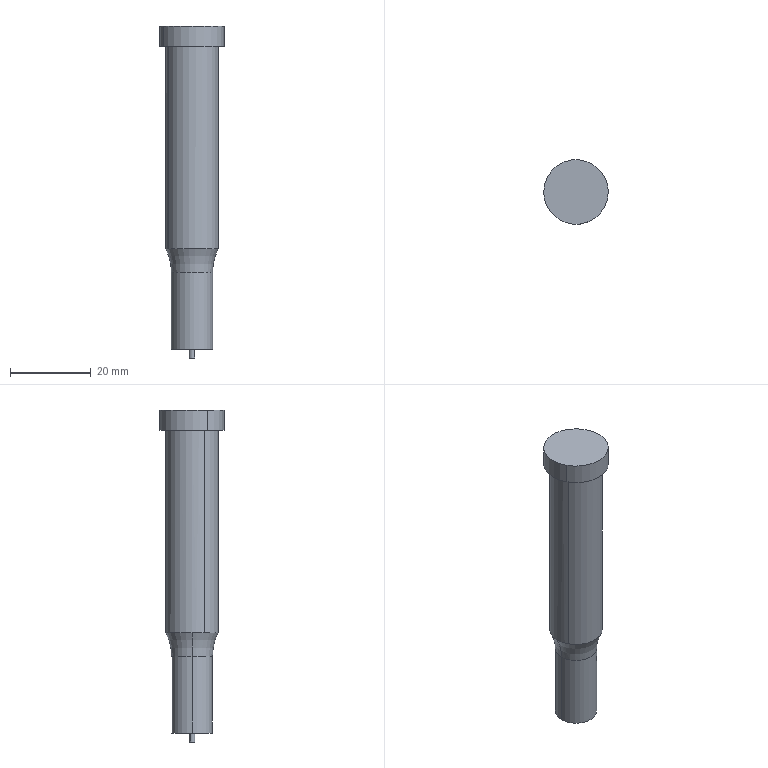Part | CATIA | 1 solid | 14 faces | box 16 x 16 x 82.2 mm | volume 9788 mm3 | cylinder 8 | plane 4 | torus 2 | commonest cylinder face diameters 1.47 x2 10.2 x2 13 x2 16 x2
STEP:
#1=CARTESIAN_POINT('',(5.1,0.,0.));
#2=VERTEX_POINT('',#1);
#3=CARTESIAN_POINT('',(-5.1,0.,0.));
#4=VERTEX_POINT('',#3);
#5=CARTESIAN_POINT('',(0.,0.,0.));
#6=DIRECTION('',(0.,0.,1.));
#7=AXIS2_PLACEMENT_3D('',#5,#6,$);
#8=CIRCLE('',#7,5.1);
#9=EDGE_CURVE('',#2,#4,#8,.T.);
#10=ORIENTED_EDGE('',*,*,#9,.F.);
#11=CARTESIAN_POINT('',(0.,0.,0.));
#12=DIRECTION('',(0.,0.,1.));
#13=AXIS2_PLACEMENT_3D('',#11,#12,$);
#14=CIRCLE('',#13,5.1);
#15=EDGE_CURVE('',#4,#2,#14,.T.);
#16=ORIENTED_EDGE('',*,*,#15,.F.);
#17=EDGE_LOOP('',(#10,#16));
#18=FACE_OUTER_BOUND('',#17,.T.);
#19=CARTESIAN_POINT('',(0.645,-0.3524,0.));
#20=VERTEX_POINT('',#19);
#21=CARTESIAN_POINT('',(-0.645,0.3524,0.));
#22=VERTEX_POINT('',#21);
#23=CARTESIAN_POINT('',(0.,0.,0.));
#24=DIRECTION('',(0.,0.,1.));
#25=AXIS2_PLACEMENT_3D('',#23,#24,$);
#26=CIRCLE('',#25,0.735);
#27=EDGE_CURVE('',#20,#22,#26,.F.);
#28=ORIENTED_EDGE('',*,*,#27,.F.);
#29=CARTESIAN_POINT('',(0.,0.,0.));
#30=DIRECTION('',(0.,0.,1.));
#31=AXIS2_PLACEMENT_3D('',#29,#30,$);
#32=CIRCLE('',#31,0.735);
#33=EDGE_CURVE('',#22,#20,#32,.F.);
#34=ORIENTED_EDGE('',*,*,#33,.F.);
#35=EDGE_LOOP('',(#28,#34));
#36=FACE_BOUND('',#35,.T.);
#37=CARTESIAN_POINT('',(6.5,0.,0.));
#38=DIRECTION('',(0.,0.,1.));
#39=DIRECTION('',(1.,0.,0.));
#40=AXIS2_PLACEMENT_3D('',#37,#38,#39);
#41=PLANE('',#40);
#42=ADVANCED_FACE('',(#18,#36),#41,.F.);
#43=CARTESIAN_POINT('',(-6.5,0.,24.869));
#44=VERTEX_POINT('',#43);
#45=CARTESIAN_POINT('',(5.704,3.116,24.869));
#46=VERTEX_POINT('',#45);
#47=CARTESIAN_POINT('',(0.,0.,24.869));
#48=DIRECTION('',(0.,0.,-1.));
#49=AXIS2_PLACEMENT_3D('',#47,#48,$);
#50=CIRCLE('',#49,6.5);
#51=EDGE_CURVE('',#44,#46,#50,.T.);
#52=ORIENTED_EDGE('',*,*,#51,.T.);
#53=CARTESIAN_POINT('',(6.5,0.,24.869));
#54=VERTEX_POINT('',#53);
#55=CARTESIAN_POINT('',(0.,0.,24.869));
#56=DIRECTION('',(0.,0.,-1.));
#57=AXIS2_PLACEMENT_3D('',#55,#56,$);
#58=CIRCLE('',#57,6.5);
#59=EDGE_CURVE('',#46,#54,#58,.T.);
#60=ORIENTED_EDGE('',*,*,#59,.T.);
#61=CARTESIAN_POINT('',(5.1,0.,19.));
#62=VERTEX_POINT('',#61);
#63=CARTESIAN_POINT('',(18.1,0.,19.));
#64=DIRECTION('',(0.,1.,0.));
#65=AXIS2_PLACEMENT_3D('',#63,#64,$);
#66=CIRCLE('',#65,13.);
#67=EDGE_CURVE('',#54,#62,#66,.F.);
#68=ORIENTED_EDGE('',*,*,#67,.T.);
#69=CARTESIAN_POINT('',(-5.1,0.,19.));
#70=VERTEX_POINT('',#69);
#71=CARTESIAN_POINT('',(0.,0.,19.));
#72=DIRECTION('',(0.,0.,-1.));
#73=AXIS2_PLACEMENT_3D('',#71,#72,$);
#74=CIRCLE('',#73,5.1);
#75=EDGE_CURVE('',#70,#62,#74,.T.);
#76=ORIENTED_EDGE('',*,*,#75,.F.);
#77=CARTESIAN_POINT('',(-18.1,0.,19.));
#78=DIRECTION('',(0.,-1.,0.));
#79=AXIS2_PLACEMENT_3D('',#77,#78,$);
#80=CIRCLE('',#79,13.);
#81=EDGE_CURVE('',#44,#70,#80,.F.);
#82=ORIENTED_EDGE('',*,*,#81,.F.);
#83=EDGE_LOOP('',(#52,#60,#68,#76,#82));
#84=FACE_OUTER_BOUND('',#83,.T.);
#85=CARTESIAN_POINT('',(0.,0.,19.));
#86=DIRECTION('',(0.,0.,-1.));
#87=DIRECTION('',(-0.9236,-0.3833,0.));
#88=AXIS2_PLACEMENT_3D('',#85,#86,#87);
#89=TOROIDAL_SURFACE('',#88,18.1,13.);
#90=ADVANCED_FACE('',(#84),#89,.F.);
#91=CARTESIAN_POINT('',(-5.704,-3.116,24.869));
#92=VERTEX_POINT('',#91);
#93=CARTESIAN_POINT('',(0.,0.,24.869));
#94=DIRECTION('',(0.,0.,-1.));
#95=AXIS2_PLACEMENT_3D('',#93,#94,$);
#96=CIRCLE('',#95,6.5);
#97=EDGE_CURVE('',#92,#54,#96,.F.);
#98=ORIENTED_EDGE('',*,*,#97,.F.);
#99=CARTESIAN_POINT('',(0.,0.,24.869));
#100=DIRECTION('',(0.,0.,-1.));
#101=AXIS2_PLACEMENT_3D('',#99,#100,$);
#102=CIRCLE('',#101,6.5);
#103=EDGE_CURVE('',#92,#44,#102,.T.);
#104=ORIENTED_EDGE('',*,*,#103,.T.);
#105=ORIENTED_EDGE('',*,*,#81,.T.);
#106=CARTESIAN_POINT('',(0.,0.,19.));
#107=DIRECTION('',(0.,0.,-1.));
#108=AXIS2_PLACEMENT_3D('',#106,#107,$);
#109=CIRCLE('',#108,5.1);
#110=EDGE_CURVE('',#62,#70,#109,.T.);
#111=ORIENTED_EDGE('',*,*,#110,.F.);
#112=ORIENTED_EDGE('',*,*,#67,.F.);
#113=EDGE_LOOP('',(#98,#104,#105,#111,#112));
#114=FACE_OUTER_BOUND('',#113,.T.);
#115=CARTESIAN_POINT('',(0.,0.,19.));
#116=DIRECTION('',(0.,0.,-1.));
#117=DIRECTION('',(0.9063,0.4226,0.));
#118=AXIS2_PLACEMENT_3D('',#115,#116,#117);
#119=TOROIDAL_SURFACE('',#118,18.1,13.);
#120=ADVANCED_FACE('',(#114),#119,.F.);
#121=CARTESIAN_POINT('',(5.1,0.,16.61));
#122=DIRECTION('',(0.,0.,1.));
#123=VECTOR('',#122,1.);
#124=LINE('',#121,#123);
#125=EDGE_CURVE('',#2,#62,#124,.T.);
#126=ORIENTED_EDGE('',*,*,#125,.F.);
#127=ORIENTED_EDGE('',*,*,#9,.T.);
#128=CARTESIAN_POINT('',(-5.1,0.,16.61));
#129=DIRECTION('',(0.,0.,1.));
#130=VECTOR('',#129,1.);
#131=LINE('',#128,#130);
#132=EDGE_CURVE('',#4,#70,#131,.T.);
#133=ORIENTED_EDGE('',*,*,#132,.T.);
#134=ORIENTED_EDGE('',*,*,#75,.T.);
#135=EDGE_LOOP('',(#126,#127,#133,#134));
#136=FACE_OUTER_BOUND('',#135,.T.);
#137=CARTESIAN_POINT('',(0.,0.,16.61));
#138=DIRECTION('',(0.,0.,1.));
#139=DIRECTION('',(1.,0.,0.));
#140=AXIS2_PLACEMENT_3D('',#137,#138,#139);
#141=CYLINDRICAL_SURFACE('',#140,5.1);
#142=ADVANCED_FACE('',(#136),#141,.T.);
#143=ORIENTED_EDGE('',*,*,#132,.F.);
#144=ORIENTED_EDGE('',*,*,#15,.T.);
#145=ORIENTED_EDGE('',*,*,#125,.T.);
#146=ORIENTED_EDGE('',*,*,#110,.T.);
#147=EDGE_LOOP('',(#143,#144,#145,#146));
#148=FACE_OUTER_BOUND('',#147,.T.);
#149=CARTESIAN_POINT('',(0.,0.,16.61));
#150=DIRECTION('',(0.,0.,1.));
#151=DIRECTION('',(-1.,0.,0.));
#152=AXIS2_PLACEMENT_3D('',#149,#150,#151);
#153=CYLINDRICAL_SURFACE('',#152,5.1);
#154=ADVANCED_FACE('',(#148),#153,.T.);
#155=CARTESIAN_POINT('',(-5.704,-3.116,75.));
#156=VERTEX_POINT('',#155);
#157=CARTESIAN_POINT('',(-5.704,-3.116,37.5));
#158=DIRECTION('',(0.,0.,1.));
#159=VECTOR('',#158,1.);
#160=LINE('',#157,#159);
#161=EDGE_CURVE('',#92,#156,#160,.T.);
#162=ORIENTED_EDGE('',*,*,#161,.T.);
#163=CARTESIAN_POINT('',(5.704,3.116,75.));
#164=VERTEX_POINT('',#163);
#165=CARTESIAN_POINT('',(0.,0.,75.));
#166=DIRECTION('',(0.,0.,1.));
#167=AXIS2_PLACEMENT_3D('',#165,#166,$);
#168=CIRCLE('',#167,6.5);
#169=EDGE_CURVE('',#164,#156,#168,.T.);
#170=ORIENTED_EDGE('',*,*,#169,.F.);
#171=CARTESIAN_POINT('',(5.704,3.116,37.5));
#172=DIRECTION('',(0.,0.,1.));
#173=VECTOR('',#172,1.);
#174=LINE('',#171,#173);
#175=EDGE_CURVE('',#46,#164,#174,.T.);
#176=ORIENTED_EDGE('',*,*,#175,.F.);
#177=ORIENTED_EDGE('',*,*,#51,.F.);
#178=ORIENTED_EDGE('',*,*,#103,.F.);
#179=EDGE_LOOP('',(#162,#170,#176,#177,#178));
#180=FACE_OUTER_BOUND('',#179,.T.);
#181=CARTESIAN_POINT('',(0.,0.,40.));
#182=DIRECTION('',(0.,0.,1.));
#183=DIRECTION('',(0.8776,0.4794,0.));
#184=AXIS2_PLACEMENT_3D('',#181,#182,#183);
#185=CYLINDRICAL_SURFACE('',#184,6.5);
#186=ADVANCED_FACE('',(#180),#185,.T.);
#187=ORIENTED_EDGE('',*,*,#175,.T.);
#188=CARTESIAN_POINT('',(0.,0.,75.));
#189=DIRECTION('',(0.,0.,1.));
#190=AXIS2_PLACEMENT_3D('',#188,#189,$);
#191=CIRCLE('',#190,6.5);
#192=EDGE_CURVE('',#156,#164,#191,.T.);
#193=ORIENTED_EDGE('',*,*,#192,.F.);
#194=ORIENTED_EDGE('',*,*,#161,.F.);
#195=ORIENTED_EDGE('',*,*,#97,.T.);
#196=ORIENTED_EDGE('',*,*,#59,.F.);
#197=EDGE_LOOP('',(#187,#193,#194,#195,#196));
#198=FACE_OUTER_BOUND('',#197,.T.);
#199=ADVANCED_FACE('',(#198),#185,.T.);
#200=CARTESIAN_POINT('',(-7.021,-3.835,80.));
#201=VERTEX_POINT('',#200);
#202=CARTESIAN_POINT('',(7.021,3.835,80.));
#203=VERTEX_POINT('',#202);
#204=CARTESIAN_POINT('',(0.,0.,80.));
#205=DIRECTION('',(0.,0.,1.));
#206=AXIS2_PLACEMENT_3D('',#204,#205,$);
#207=CIRCLE('',#206,8.);
#208=EDGE_CURVE('',#201,#203,#207,.T.);
#209=ORIENTED_EDGE('',*,*,#208,.T.);
#210=CARTESIAN_POINT('',(0.,0.,80.));
#211=DIRECTION('',(0.,0.,1.));
#212=AXIS2_PLACEMENT_3D('',#210,#211,$);
#213=CIRCLE('',#212,8.);
#214=EDGE_CURVE('',#203,#201,#213,.T.);
#215=ORIENTED_EDGE('',*,*,#214,.T.);
#216=EDGE_LOOP('',(#209,#215));
#217=FACE_OUTER_BOUND('',#216,.T.);
#218=CARTESIAN_POINT('',(0.,0.,80.));
#219=DIRECTION('',(0.,0.,1.));
#220=DIRECTION('',(1.,0.,0.));
#221=AXIS2_PLACEMENT_3D('',#218,#219,#220);
#222=PLANE('',#221);
#223=ADVANCED_FACE('',(#217),#222,.T.);
#224=CARTESIAN_POINT('',(7.021,3.835,75.));
#225=VERTEX_POINT('',#224);
#226=CARTESIAN_POINT('',(-7.021,-3.835,75.));
#227=VERTEX_POINT('',#226);
#228=CARTESIAN_POINT('',(0.,0.,75.));
#229=DIRECTION('',(0.,0.,1.));
#230=AXIS2_PLACEMENT_3D('',#228,#229,$);
#231=CIRCLE('',#230,8.);
#232=EDGE_CURVE('',#225,#227,#231,.T.);
#233=ORIENTED_EDGE('',*,*,#232,.F.);
#234=CARTESIAN_POINT('',(0.,0.,75.));
#235=DIRECTION('',(0.,0.,1.));
#236=AXIS2_PLACEMENT_3D('',#234,#235,$);
#237=CIRCLE('',#236,8.);
#238=EDGE_CURVE('',#227,#225,#237,.T.);
#239=ORIENTED_EDGE('',*,*,#238,.F.);
#240=EDGE_LOOP('',(#233,#239));
#241=FACE_OUTER_BOUND('',#240,.T.);
#242=ORIENTED_EDGE('',*,*,#192,.T.);
#243=ORIENTED_EDGE('',*,*,#169,.T.);
#244=EDGE_LOOP('',(#242,#243));
#245=FACE_BOUND('',#244,.T.);
#246=CARTESIAN_POINT('',(8.,0.,75.));
#247=DIRECTION('',(0.,0.,1.));
#248=DIRECTION('',(1.,0.,0.));
#249=AXIS2_PLACEMENT_3D('',#246,#247,#248);
#250=PLANE('',#249);
#251=ADVANCED_FACE('',(#241,#245),#250,.F.);
#252=CARTESIAN_POINT('',(7.021,3.835,77.5));
#253=DIRECTION('',(0.,0.,1.));
#254=VECTOR('',#253,1.);
#255=LINE('',#252,#254);
#256=EDGE_CURVE('',#225,#203,#255,.T.);
#257=ORIENTED_EDGE('',*,*,#256,.T.);
#258=ORIENTED_EDGE('',*,*,#208,.F.);
#259=CARTESIAN_POINT('',(-7.021,-3.835,77.5));
#260=DIRECTION('',(0.,0.,1.));
#261=VECTOR('',#260,1.);
#262=LINE('',#259,#261);
#263=EDGE_CURVE('',#227,#201,#262,.T.);
#264=ORIENTED_EDGE('',*,*,#263,.F.);
#265=ORIENTED_EDGE('',*,*,#238,.T.);
#266=EDGE_LOOP('',(#257,#258,#264,#265));
#267=FACE_OUTER_BOUND('',#266,.T.);
#268=CARTESIAN_POINT('',(0.,0.,40.));
#269=DIRECTION('',(0.,0.,1.));
#270=DIRECTION('',(0.8776,0.4794,0.));
#271=AXIS2_PLACEMENT_3D('',#268,#269,#270);
#272=CYLINDRICAL_SURFACE('',#271,8.);
#273=ADVANCED_FACE('',(#267),#272,.T.);
#274=ORIENTED_EDGE('',*,*,#263,.T.);
#275=ORIENTED_EDGE('',*,*,#214,.F.);
#276=ORIENTED_EDGE('',*,*,#256,.F.);
#277=ORIENTED_EDGE('',*,*,#232,.T.);
#278=EDGE_LOOP('',(#274,#275,#276,#277));
#279=FACE_OUTER_BOUND('',#278,.T.);
#280=ADVANCED_FACE('',(#279),#272,.T.);
#281=CARTESIAN_POINT('',(0.645,-0.3524,-2.2));
#282=VERTEX_POINT('',#281);
#283=CARTESIAN_POINT('',(-0.645,0.3524,-2.2));
#284=VERTEX_POINT('',#283);
#285=CARTESIAN_POINT('',(0.,0.,-2.2));
#286=DIRECTION('',(0.,0.,-1.));
#287=AXIS2_PLACEMENT_3D('',#285,#286,$);
#288=CIRCLE('',#287,0.735);
#289=EDGE_CURVE('',#282,#284,#288,.T.);
#290=ORIENTED_EDGE('',*,*,#289,.F.);
#291=CARTESIAN_POINT('',(0.645,-0.3524,-1.1));
#292=DIRECTION('',(0.,0.,-1.));
#293=VECTOR('',#292,1.);
#294=LINE('',#291,#293);
#295=EDGE_CURVE('',#282,#20,#294,.F.);
#296=ORIENTED_EDGE('',*,*,#295,.T.);
#297=ORIENTED_EDGE('',*,*,#27,.T.);
#298=CARTESIAN_POINT('',(-0.645,0.3524,-1.1));
#299=DIRECTION('',(0.,0.,-1.));
#300=VECTOR('',#299,1.);
#301=LINE('',#298,#300);
#302=EDGE_CURVE('',#284,#22,#301,.F.);
#303=ORIENTED_EDGE('',*,*,#302,.F.);
#304=EDGE_LOOP('',(#290,#296,#297,#303));
#305=FACE_OUTER_BOUND('',#304,.T.);
#306=CARTESIAN_POINT('',(0.,0.,-1.1));
#307=DIRECTION('',(0.,0.,-1.));
#308=DIRECTION('',(0.8776,-0.4794,0.));
#309=AXIS2_PLACEMENT_3D('',#306,#307,#308);
#310=CYLINDRICAL_SURFACE('',#309,0.735);
#311=ADVANCED_FACE('',(#305),#310,.T.);
#312=CARTESIAN_POINT('',(0.,0.,-2.2));
#313=DIRECTION('',(0.,0.,-1.));
#314=AXIS2_PLACEMENT_3D('',#312,#313,$);
#315=CIRCLE('',#314,0.735);
#316=EDGE_CURVE('',#284,#282,#315,.T.);
#317=ORIENTED_EDGE('',*,*,#316,.F.);
#318=ORIENTED_EDGE('',*,*,#302,.T.);
#319=ORIENTED_EDGE('',*,*,#33,.T.);
#320=ORIENTED_EDGE('',*,*,#295,.F.);
#321=EDGE_LOOP('',(#317,#318,#319,#320));
#322=FACE_OUTER_BOUND('',#321,.T.);
#323=ADVANCED_FACE('',(#322),#310,.T.);
#324=ORIENTED_EDGE('',*,*,#289,.T.);
#325=ORIENTED_EDGE('',*,*,#316,.T.);
#326=EDGE_LOOP('',(#324,#325));
#327=FACE_OUTER_BOUND('',#326,.T.);
#328=CARTESIAN_POINT('',(0.735,0.,-2.2));
#329=DIRECTION('',(0.,0.,-1.));
#330=DIRECTION('',(1.,0.,0.));
#331=AXIS2_PLACEMENT_3D('',#328,#329,#330);
#332=PLANE('',#331);
#333=ADVANCED_FACE('',(#327),#332,.T.);
#334=CLOSED_SHELL('',(#42,#90,#120,#142,#154,#186,#199,#223,#251,#273,#280,#311,#323,#333));
#335=MANIFOLD_SOLID_BREP('',#334);
#336=(LENGTH_UNIT()NAMED_UNIT(*)SI_UNIT(.MILLI.,.METRE.));
#337=UNCERTAINTY_MEASURE_WITH_UNIT(LENGTH_MEASURE(0.005),#336,'','');
#338=(NAMED_UNIT(*)PLANE_ANGLE_UNIT()SI_UNIT($,.RADIAN.));
#339=(NAMED_UNIT(*)SI_UNIT($,.STERADIAN.)SOLID_ANGLE_UNIT());
#340=(GEOMETRIC_REPRESENTATION_CONTEXT(3)GLOBAL_UNCERTAINTY_ASSIGNED_CONTEXT((#337))GLOBAL_UNIT_ASSIGNED_CONTEXT((#336,#338,#339))REPRESENTATION_CONTEXT('',''));
#341=ADVANCED_BREP_SHAPE_REPRESENTATION('',(#335),#340);